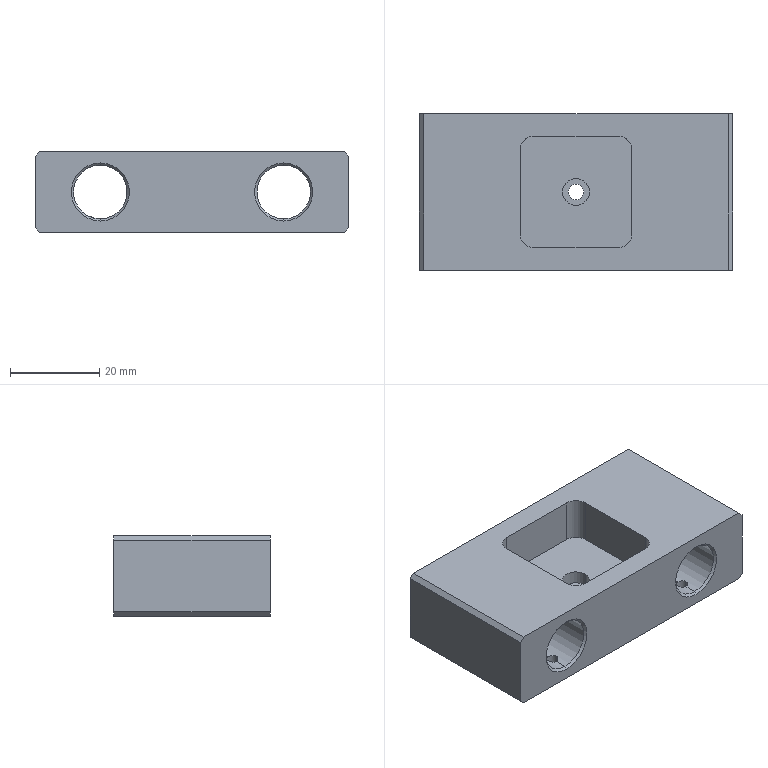Part | SolidWorks | features ICE 3, Chamfer 2, HoleWzd 2, Extrusion 1 | 1 solid | 47 faces | box 70 x 35 x 18 mm | volume 29673 mm3 | cylinder 22 | plane 17 | cone 8 | commonest cylinder face diameters 2.5 x8 6 x8 12 x4 3.5 x2